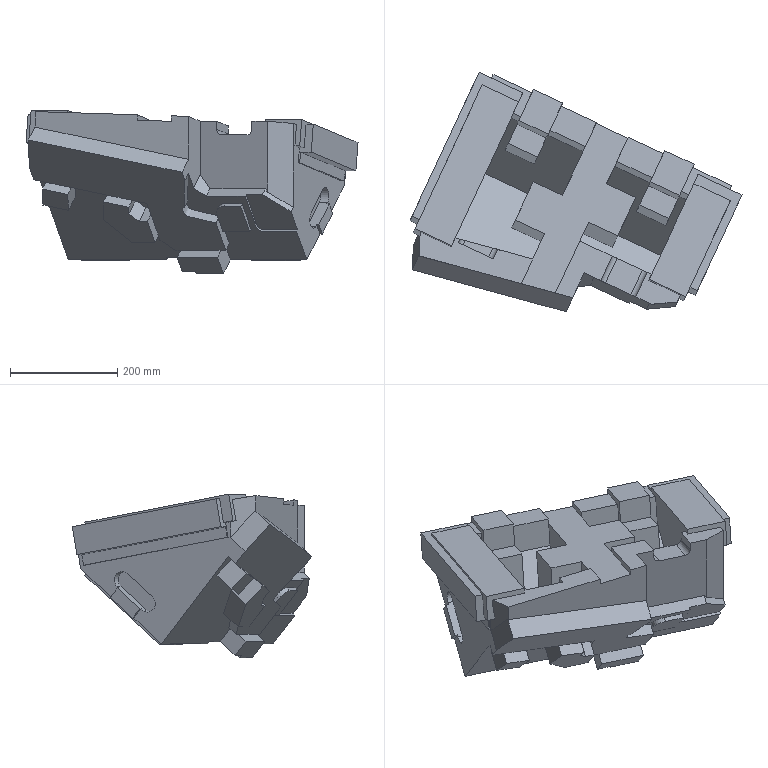Part | NX | features solid 2 | 1 solid | 177 faces | box 618.155 x 445.546 x 304.621 mm | volume 21433051 mm3 | plane 163 | cylinder 12 | spline 2 | commonest cylinder face diameters 20 x6 32 x4 15 x1 40 x1